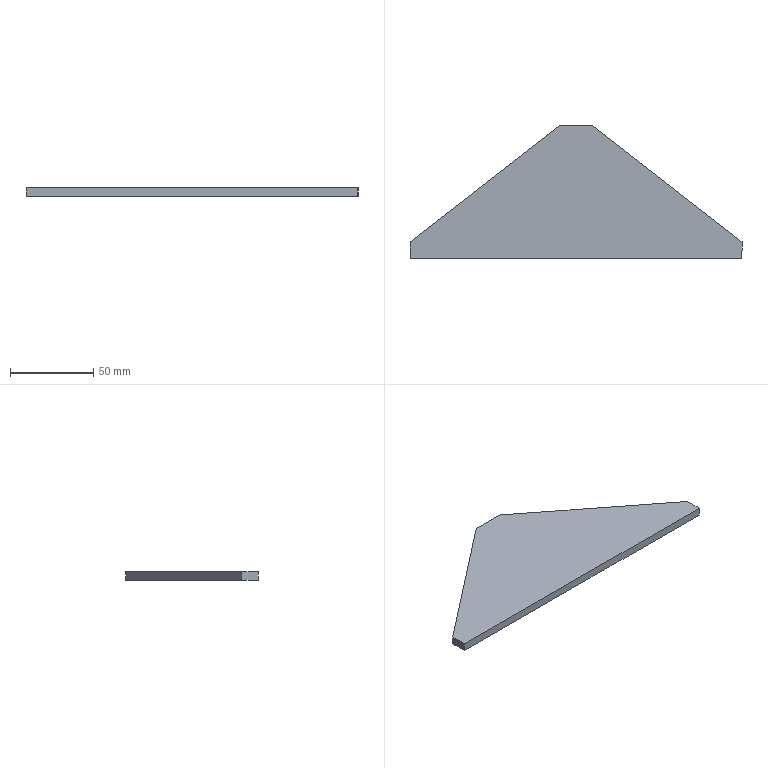Part | SolidWorks | features Extrusion 1 | 1 solid | 8 faces | box 200 x 80 x 5 mm | volume 48500 mm3 | plane 8
STEP:
#1=CARTESIAN_POINT('',(100.,-59.77,0.));
#2=VERTEX_POINT('',#1);
#3=CARTESIAN_POINT('',(100.,-49.77,0.));
#4=VERTEX_POINT('',#3);
#5=CARTESIAN_POINT('',(100.,-49.77,0.));
#6=DIRECTION('',(0.,1.,0.));
#7=VECTOR('',#6,1000.);
#8=LINE('',#5,#7);
#9=EDGE_CURVE('',#2,#4,#8,.T.);
#10=ORIENTED_EDGE('',*,*,#9,.T.);
#11=CARTESIAN_POINT('',(100.,-49.77,5.));
#12=VERTEX_POINT('',#11);
#13=CARTESIAN_POINT('',(100.,-49.77,5.));
#14=DIRECTION('',(0.,0.,-1.));
#15=VECTOR('',#14,1000.);
#16=LINE('',#13,#15);
#17=EDGE_CURVE('',#12,#4,#16,.T.);
#18=ORIENTED_EDGE('',*,*,#17,.F.);
#19=CARTESIAN_POINT('',(100.,-59.77,5.));
#20=VERTEX_POINT('',#19);
#21=CARTESIAN_POINT('',(100.,-49.77,5.));
#22=DIRECTION('',(0.,1.,0.));
#23=VECTOR('',#22,1000.);
#24=LINE('',#21,#23);
#25=EDGE_CURVE('',#20,#12,#24,.T.);
#26=ORIENTED_EDGE('',*,*,#25,.F.);
#27=CARTESIAN_POINT('',(100.,-59.77,5.));
#28=DIRECTION('',(0.,0.,-1.));
#29=VECTOR('',#28,1000.);
#30=LINE('',#27,#29);
#31=EDGE_CURVE('',#20,#2,#30,.T.);
#32=ORIENTED_EDGE('',*,*,#31,.T.);
#33=EDGE_LOOP('',(#10,#18,#26,#32));
#34=FACE_OUTER_BOUND('',#33,.T.);
#35=CARTESIAN_POINT('',(100.,-49.77,5.));
#36=DIRECTION('',(-1.,0.,0.));
#37=DIRECTION('',(0.,-1.,0.));
#38=AXIS2_PLACEMENT_3D('',#35,#36,#37);
#39=PLANE('',#38);
#40=ADVANCED_FACE('',(#34),#39,.F.);
#41=CARTESIAN_POINT('',(10.,20.23,0.));
#42=VERTEX_POINT('',#41);
#43=CARTESIAN_POINT('',(10.,20.23,0.));
#44=DIRECTION('',(-0.7894,0.6139,0.));
#45=VECTOR('',#44,1000.);
#46=LINE('',#43,#45);
#47=EDGE_CURVE('',#4,#42,#46,.T.);
#48=ORIENTED_EDGE('',*,*,#47,.T.);
#49=CARTESIAN_POINT('',(10.,20.23,5.));
#50=VERTEX_POINT('',#49);
#51=CARTESIAN_POINT('',(10.,20.23,5.));
#52=DIRECTION('',(0.,0.,-1.));
#53=VECTOR('',#52,1000.);
#54=LINE('',#51,#53);
#55=EDGE_CURVE('',#50,#42,#54,.T.);
#56=ORIENTED_EDGE('',*,*,#55,.F.);
#57=CARTESIAN_POINT('',(10.,20.23,5.));
#58=DIRECTION('',(-0.7894,0.6139,0.));
#59=VECTOR('',#58,1000.);
#60=LINE('',#57,#59);
#61=EDGE_CURVE('',#12,#50,#60,.T.);
#62=ORIENTED_EDGE('',*,*,#61,.F.);
#63=ORIENTED_EDGE('',*,*,#17,.T.);
#64=EDGE_LOOP('',(#48,#56,#62,#63));
#65=FACE_OUTER_BOUND('',#64,.T.);
#66=CARTESIAN_POINT('',(10.,20.23,5.));
#67=DIRECTION('',(-0.6139,-0.7894,0.));
#68=DIRECTION('',(0.7894,-0.6139,0.));
#69=AXIS2_PLACEMENT_3D('',#66,#67,#68);
#70=PLANE('',#69);
#71=ADVANCED_FACE('',(#65),#70,.F.);
#72=CARTESIAN_POINT('',(-10.,20.23,0.));
#73=VERTEX_POINT('',#72);
#74=CARTESIAN_POINT('',(-10.,20.23,0.));
#75=DIRECTION('',(-1.,0.,0.));
#76=VECTOR('',#75,1000.);
#77=LINE('',#74,#76);
#78=EDGE_CURVE('',#42,#73,#77,.T.);
#79=ORIENTED_EDGE('',*,*,#78,.T.);
#80=CARTESIAN_POINT('',(-10.,20.23,5.));
#81=VERTEX_POINT('',#80);
#82=CARTESIAN_POINT('',(-10.,20.23,5.));
#83=DIRECTION('',(0.,0.,-1.));
#84=VECTOR('',#83,1000.);
#85=LINE('',#82,#84);
#86=EDGE_CURVE('',#81,#73,#85,.T.);
#87=ORIENTED_EDGE('',*,*,#86,.F.);
#88=CARTESIAN_POINT('',(-10.,20.23,5.));
#89=DIRECTION('',(-1.,0.,0.));
#90=VECTOR('',#89,1000.);
#91=LINE('',#88,#90);
#92=EDGE_CURVE('',#50,#81,#91,.T.);
#93=ORIENTED_EDGE('',*,*,#92,.F.);
#94=ORIENTED_EDGE('',*,*,#55,.T.);
#95=EDGE_LOOP('',(#79,#87,#93,#94));
#96=FACE_OUTER_BOUND('',#95,.T.);
#97=CARTESIAN_POINT('',(-10.,20.23,5.));
#98=DIRECTION('',(0.,-1.,0.));
#99=DIRECTION('',(0.,0.,-1.));
#100=AXIS2_PLACEMENT_3D('',#97,#98,#99);
#101=PLANE('',#100);
#102=ADVANCED_FACE('',(#96),#101,.F.);
#103=CARTESIAN_POINT('',(-100.,-49.77,0.));
#104=VERTEX_POINT('',#103);
#105=CARTESIAN_POINT('',(-10.,20.23,0.));
#106=DIRECTION('',(-0.7894,-0.6139,0.));
#107=VECTOR('',#106,1000.);
#108=LINE('',#105,#107);
#109=EDGE_CURVE('',#73,#104,#108,.T.);
#110=ORIENTED_EDGE('',*,*,#109,.T.);
#111=CARTESIAN_POINT('',(-100.,-49.77,5.));
#112=VERTEX_POINT('',#111);
#113=CARTESIAN_POINT('',(-100.,-49.77,5.));
#114=DIRECTION('',(0.,0.,-1.));
#115=VECTOR('',#114,1000.);
#116=LINE('',#113,#115);
#117=EDGE_CURVE('',#112,#104,#116,.T.);
#118=ORIENTED_EDGE('',*,*,#117,.F.);
#119=CARTESIAN_POINT('',(-10.,20.23,5.));
#120=DIRECTION('',(-0.7894,-0.6139,0.));
#121=VECTOR('',#120,1000.);
#122=LINE('',#119,#121);
#123=EDGE_CURVE('',#81,#112,#122,.T.);
#124=ORIENTED_EDGE('',*,*,#123,.F.);
#125=ORIENTED_EDGE('',*,*,#86,.T.);
#126=EDGE_LOOP('',(#110,#118,#124,#125));
#127=FACE_OUTER_BOUND('',#126,.T.);
#128=CARTESIAN_POINT('',(-10.,20.23,5.));
#129=DIRECTION('',(0.6139,-0.7894,0.));
#130=DIRECTION('',(0.7894,0.6139,0.));
#131=AXIS2_PLACEMENT_3D('',#128,#129,#130);
#132=PLANE('',#131);
#133=ADVANCED_FACE('',(#127),#132,.F.);
#134=CARTESIAN_POINT('',(-100.,-59.77,0.));
#135=VERTEX_POINT('',#134);
#136=CARTESIAN_POINT('',(-100.,-49.77,0.));
#137=DIRECTION('',(0.,-1.,0.));
#138=VECTOR('',#137,1000.);
#139=LINE('',#136,#138);
#140=EDGE_CURVE('',#104,#135,#139,.T.);
#141=ORIENTED_EDGE('',*,*,#140,.T.);
#142=CARTESIAN_POINT('',(-100.,-59.77,5.));
#143=VERTEX_POINT('',#142);
#144=CARTESIAN_POINT('',(-100.,-59.77,5.));
#145=DIRECTION('',(0.,0.,-1.));
#146=VECTOR('',#145,1000.);
#147=LINE('',#144,#146);
#148=EDGE_CURVE('',#143,#135,#147,.T.);
#149=ORIENTED_EDGE('',*,*,#148,.F.);
#150=CARTESIAN_POINT('',(-100.,-49.77,5.));
#151=DIRECTION('',(0.,-1.,0.));
#152=VECTOR('',#151,1000.);
#153=LINE('',#150,#152);
#154=EDGE_CURVE('',#112,#143,#153,.T.);
#155=ORIENTED_EDGE('',*,*,#154,.F.);
#156=ORIENTED_EDGE('',*,*,#117,.T.);
#157=EDGE_LOOP('',(#141,#149,#155,#156));
#158=FACE_OUTER_BOUND('',#157,.T.);
#159=CARTESIAN_POINT('',(-100.,-49.77,5.));
#160=DIRECTION('',(1.,0.,0.));
#161=DIRECTION('',(0.,1.,0.));
#162=AXIS2_PLACEMENT_3D('',#159,#160,#161);
#163=PLANE('',#162);
#164=ADVANCED_FACE('',(#158),#163,.F.);
#165=CARTESIAN_POINT('',(-100.,-59.77,0.));
#166=DIRECTION('',(1.,0.,0.));
#167=VECTOR('',#166,1000.);
#168=LINE('',#165,#167);
#169=EDGE_CURVE('',#135,#2,#168,.T.);
#170=ORIENTED_EDGE('',*,*,#169,.T.);
#171=ORIENTED_EDGE('',*,*,#31,.F.);
#172=CARTESIAN_POINT('',(-100.,-59.77,5.));
#173=DIRECTION('',(1.,0.,0.));
#174=VECTOR('',#173,1000.);
#175=LINE('',#172,#174);
#176=EDGE_CURVE('',#143,#20,#175,.T.);
#177=ORIENTED_EDGE('',*,*,#176,.F.);
#178=ORIENTED_EDGE('',*,*,#148,.T.);
#179=EDGE_LOOP('',(#170,#171,#177,#178));
#180=FACE_OUTER_BOUND('',#179,.T.);
#181=CARTESIAN_POINT('',(-100.,-59.77,5.));
#182=DIRECTION('',(0.,1.,0.));
#183=DIRECTION('',(0.,0.,1.));
#184=AXIS2_PLACEMENT_3D('',#181,#182,#183);
#185=PLANE('',#184);
#186=ADVANCED_FACE('',(#180),#185,.F.);
#187=ORIENTED_EDGE('',*,*,#25,.T.);
#188=ORIENTED_EDGE('',*,*,#61,.T.);
#189=ORIENTED_EDGE('',*,*,#92,.T.);
#190=ORIENTED_EDGE('',*,*,#123,.T.);
#191=ORIENTED_EDGE('',*,*,#154,.T.);
#192=ORIENTED_EDGE('',*,*,#176,.T.);
#193=EDGE_LOOP('',(#187,#188,#189,#190,#191,#192));
#194=FACE_OUTER_BOUND('',#193,.T.);
#195=CARTESIAN_POINT('',(0.,0.,5.));
#196=DIRECTION('',(0.,0.,1.));
#197=DIRECTION('',(1.,0.,0.));
#198=AXIS2_PLACEMENT_3D('',#195,#196,#197);
#199=PLANE('',#198);
#200=ADVANCED_FACE('',(#194),#199,.T.);
#201=ORIENTED_EDGE('',*,*,#9,.F.);
#202=ORIENTED_EDGE('',*,*,#169,.F.);
#203=ORIENTED_EDGE('',*,*,#140,.F.);
#204=ORIENTED_EDGE('',*,*,#109,.F.);
#205=ORIENTED_EDGE('',*,*,#78,.F.);
#206=ORIENTED_EDGE('',*,*,#47,.F.);
#207=EDGE_LOOP('',(#201,#202,#203,#204,#205,#206));
#208=FACE_OUTER_BOUND('',#207,.T.);
#209=CARTESIAN_POINT('',(0.,0.,0.));
#210=DIRECTION('',(0.,0.,1.));
#211=DIRECTION('',(1.,0.,0.));
#212=AXIS2_PLACEMENT_3D('',#209,#210,#211);
#213=PLANE('',#212);
#214=ADVANCED_FACE('',(#208),#213,.F.);
#215=CLOSED_SHELL('',(#40,#71,#102,#133,#164,#186,#200,#214));
#216=MANIFOLD_SOLID_BREP('',#215);
#217=CARTESIAN_POINT('',(0.,0.,0.));
#218=DIRECTION('',(0.,0.,1.));
#219=DIRECTION('',(1.,0.,0.));
#220=AXIS2_PLACEMENT_3D('',#217,#218,#219);
#221=(LENGTH_UNIT()NAMED_UNIT(*)SI_UNIT(.MILLI.,.METRE.));
#222=UNCERTAINTY_MEASURE_WITH_UNIT(LENGTH_MEASURE(0.00001),#221,'','');
#223=(NAMED_UNIT(*)PLANE_ANGLE_UNIT()SI_UNIT($,.RADIAN.));
#224=(NAMED_UNIT(*)SI_UNIT($,.STERADIAN.)SOLID_ANGLE_UNIT());
#225=(GEOMETRIC_REPRESENTATION_CONTEXT(3)GLOBAL_UNCERTAINTY_ASSIGNED_CONTEXT((#222))GLOBAL_UNIT_ASSIGNED_CONTEXT((#221,#223,#224))REPRESENTATION_CONTEXT('',''));
#226=ADVANCED_BREP_SHAPE_REPRESENTATION('',(#216,#220),#225);